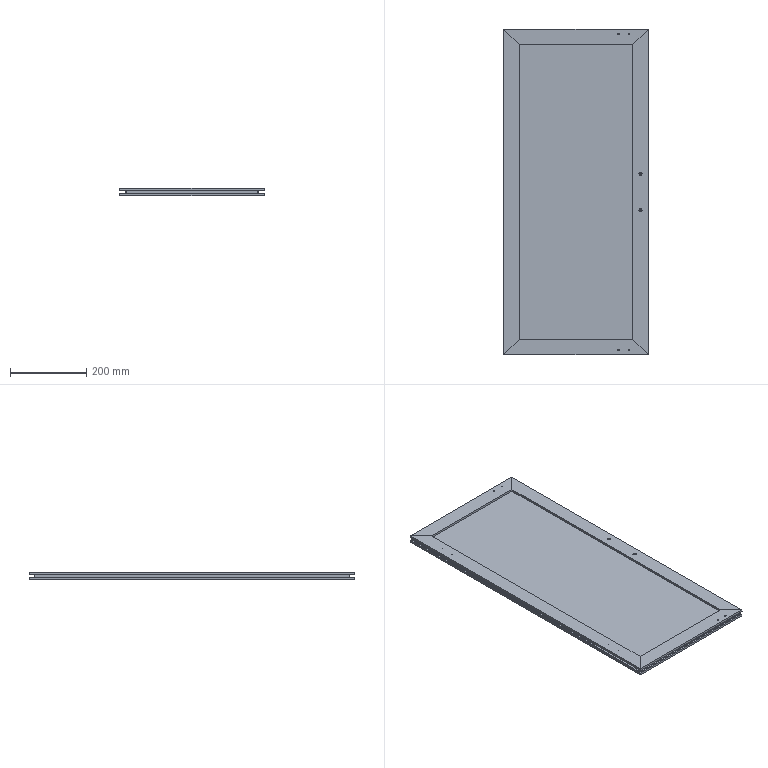Part | SolidWorks | features HoleWzd 3, ICE 1, WeldMemberFeat 1, WeldmentFeature 1 | 5 solids | 184 faces | box 379.5 x 856 x 20 mm | volume 2107206 mm3 | plane 132 | cylinder 44 | cone 8 | commonest cylinder face diameters 5 x16 3.3 x8 4.5 x8 6.5 x8 8 x4